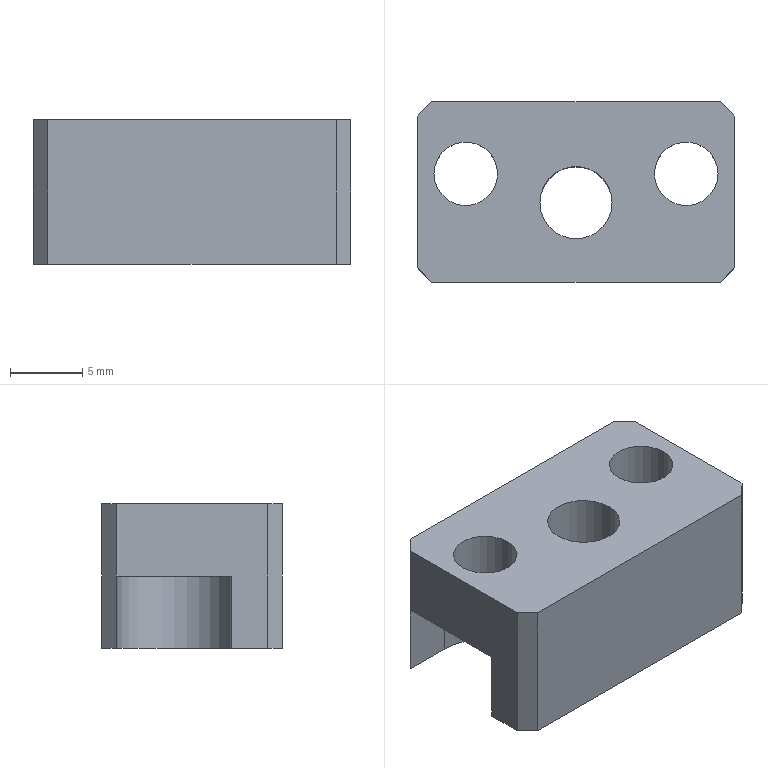Part | SolidWorks | features HoleWzd 2, ICE 2, Chamfer 1, Extrusion 1, MoveFace 1 | 1 solid | 25 faces | box 22 x 12.5 x 10 mm | volume 1861 mm3 | plane 16 | cylinder 9 | commonest cylinder face diameters 4.4 x4 8 x3 5 x2
STEP:
#1=CARTESIAN_POINT('',(5.43,0.,10.));
#2=VERTEX_POINT('',#1);
#3=CARTESIAN_POINT('',(9.83,0.,10.));
#4=VERTEX_POINT('',#3);
#5=CARTESIAN_POINT('',(7.63,0.,10.));
#6=DIRECTION('',(0.,0.,1.));
#7=DIRECTION('',(1.,0.,0.));
#8=AXIS2_PLACEMENT_3D('',#5,#6,#7);
#9=CIRCLE('',#8,2.2);
#10=EDGE_CURVE('',#2,#4,#9,.T.);
#11=ORIENTED_EDGE('',*,*,#10,.T.);
#12=CARTESIAN_POINT('',(9.83,0.,5.));
#13=VERTEX_POINT('',#12);
#14=CARTESIAN_POINT('',(9.83,0.,0.));
#15=DIRECTION('',(0.,0.,-1.));
#16=VECTOR('',#15,1000.);
#17=LINE('',#14,#16);
#18=EDGE_CURVE('',#4,#13,#17,.T.);
#19=ORIENTED_EDGE('',*,*,#18,.T.);
#20=CARTESIAN_POINT('',(5.43,0.,5.));
#21=VERTEX_POINT('',#20);
#22=CARTESIAN_POINT('',(7.63,0.,5.));
#23=DIRECTION('',(0.,0.,-1.));
#24=DIRECTION('',(-1.,0.,0.));
#25=AXIS2_PLACEMENT_3D('',#22,#23,#24);
#26=CIRCLE('',#25,2.2);
#27=EDGE_CURVE('',#13,#21,#26,.T.);
#28=ORIENTED_EDGE('',*,*,#27,.T.);
#29=CARTESIAN_POINT('',(5.43,0.,0.));
#30=DIRECTION('',(0.,0.,-1.));
#31=VECTOR('',#30,1000.);
#32=LINE('',#29,#31);
#33=EDGE_CURVE('',#2,#21,#32,.T.);
#34=ORIENTED_EDGE('',*,*,#33,.F.);
#35=EDGE_LOOP('',(#11,#19,#28,#34));
#36=FACE_OUTER_BOUND('',#35,.T.);
#37=CARTESIAN_POINT('',(7.63,0.,0.));
#38=DIRECTION('',(0.,0.,-1.));
#39=DIRECTION('',(-1.,0.,0.));
#40=AXIS2_PLACEMENT_3D('',#37,#38,#39);
#41=CYLINDRICAL_SURFACE('',#40,2.2);
#42=ADVANCED_FACE('',(#36),#41,.F.);
#43=CARTESIAN_POINT('',(-9.83,0.,10.));
#44=VERTEX_POINT('',#43);
#45=CARTESIAN_POINT('',(-5.43,0.,10.));
#46=VERTEX_POINT('',#45);
#47=CARTESIAN_POINT('',(-7.63,0.,10.));
#48=DIRECTION('',(0.,0.,1.));
#49=DIRECTION('',(1.,0.,0.));
#50=AXIS2_PLACEMENT_3D('',#47,#48,#49);
#51=CIRCLE('',#50,2.2);
#52=EDGE_CURVE('',#44,#46,#51,.T.);
#53=ORIENTED_EDGE('',*,*,#52,.T.);
#54=CARTESIAN_POINT('',(-5.43,0.,5.));
#55=VERTEX_POINT('',#54);
#56=CARTESIAN_POINT('',(-5.43,0.,0.));
#57=DIRECTION('',(0.,0.,-1.));
#58=VECTOR('',#57,1000.);
#59=LINE('',#56,#58);
#60=EDGE_CURVE('',#46,#55,#59,.T.);
#61=ORIENTED_EDGE('',*,*,#60,.T.);
#62=CARTESIAN_POINT('',(-9.83,0.,5.));
#63=VERTEX_POINT('',#62);
#64=CARTESIAN_POINT('',(-7.63,0.,5.));
#65=DIRECTION('',(0.,0.,-1.));
#66=DIRECTION('',(-1.,0.,0.));
#67=AXIS2_PLACEMENT_3D('',#64,#65,#66);
#68=CIRCLE('',#67,2.2);
#69=EDGE_CURVE('',#55,#63,#68,.T.);
#70=ORIENTED_EDGE('',*,*,#69,.T.);
#71=CARTESIAN_POINT('',(-9.83,0.,0.));
#72=DIRECTION('',(0.,0.,-1.));
#73=VECTOR('',#72,1000.);
#74=LINE('',#71,#73);
#75=EDGE_CURVE('',#44,#63,#74,.T.);
#76=ORIENTED_EDGE('',*,*,#75,.F.);
#77=EDGE_LOOP('',(#53,#61,#70,#76));
#78=FACE_OUTER_BOUND('',#77,.T.);
#79=CARTESIAN_POINT('',(-7.63,0.,0.));
#80=DIRECTION('',(0.,0.,-1.));
#81=DIRECTION('',(-1.,0.,0.));
#82=AXIS2_PLACEMENT_3D('',#79,#80,#81);
#83=CYLINDRICAL_SURFACE('',#82,2.2);
#84=ADVANCED_FACE('',(#78),#83,.F.);
#85=CARTESIAN_POINT('',(-2.5,-2.,0.));
#86=VERTEX_POINT('',#85);
#87=CARTESIAN_POINT('',(2.5,-2.,0.));
#88=VERTEX_POINT('',#87);
#89=CARTESIAN_POINT('',(0.,-2.,0.));
#90=DIRECTION('',(0.,0.,1.));
#91=DIRECTION('',(1.,0.,0.));
#92=AXIS2_PLACEMENT_3D('',#89,#90,#91);
#93=CIRCLE('',#92,2.5);
#94=EDGE_CURVE('',#86,#88,#93,.T.);
#95=ORIENTED_EDGE('',*,*,#94,.F.);
#96=CARTESIAN_POINT('',(-2.5,-2.,10.));
#97=VERTEX_POINT('',#96);
#98=CARTESIAN_POINT('',(-2.5,-2.,10.));
#99=DIRECTION('',(0.,0.,1.));
#100=VECTOR('',#99,1000.);
#101=LINE('',#98,#100);
#102=EDGE_CURVE('',#86,#97,#101,.T.);
#103=ORIENTED_EDGE('',*,*,#102,.T.);
#104=CARTESIAN_POINT('',(2.5,-2.,10.));
#105=VERTEX_POINT('',#104);
#106=CARTESIAN_POINT('',(0.,-2.,10.));
#107=DIRECTION('',(0.,0.,1.));
#108=DIRECTION('',(1.,0.,0.));
#109=AXIS2_PLACEMENT_3D('',#106,#107,#108);
#110=CIRCLE('',#109,2.5);
#111=EDGE_CURVE('',#97,#105,#110,.T.);
#112=ORIENTED_EDGE('',*,*,#111,.T.);
#113=CARTESIAN_POINT('',(2.5,-2.,10.));
#114=DIRECTION('',(0.,0.,1.));
#115=VECTOR('',#114,1000.);
#116=LINE('',#113,#115);
#117=EDGE_CURVE('',#88,#105,#116,.T.);
#118=ORIENTED_EDGE('',*,*,#117,.F.);
#119=EDGE_LOOP('',(#95,#103,#112,#118));
#120=FACE_OUTER_BOUND('',#119,.T.);
#121=CARTESIAN_POINT('',(0.,-2.,10.));
#122=DIRECTION('',(0.,0.,1.));
#123=DIRECTION('',(1.,0.,0.));
#124=AXIS2_PLACEMENT_3D('',#121,#122,#123);
#125=CYLINDRICAL_SURFACE('',#124,2.5);
#126=ADVANCED_FACE('',(#120),#125,.F.);
#127=CARTESIAN_POINT('',(3.63,0.,5.));
#128=VERTEX_POINT('',#127);
#129=CARTESIAN_POINT('',(7.63,4.,5.));
#130=VERTEX_POINT('',#129);
#131=CARTESIAN_POINT('',(7.63,0.,5.));
#132=DIRECTION('',(0.,0.,-1.));
#133=DIRECTION('',(-1.,0.,0.));
#134=AXIS2_PLACEMENT_3D('',#131,#132,#133);
#135=CIRCLE('',#134,4.);
#136=EDGE_CURVE('',#128,#130,#135,.T.);
#137=ORIENTED_EDGE('',*,*,#136,.F.);
#138=CARTESIAN_POINT('',(3.63,0.,0.));
#139=VERTEX_POINT('',#138);
#140=CARTESIAN_POINT('',(3.63,0.,0.));
#141=DIRECTION('',(0.,0.,-1.));
#142=VECTOR('',#141,1000.);
#143=LINE('',#140,#142);
#144=EDGE_CURVE('',#128,#139,#143,.T.);
#145=ORIENTED_EDGE('',*,*,#144,.T.);
#146=CARTESIAN_POINT('',(7.63,4.,0.));
#147=VERTEX_POINT('',#146);
#148=CARTESIAN_POINT('',(7.63,0.,0.));
#149=DIRECTION('',(0.,0.,-1.));
#150=DIRECTION('',(-1.,0.,0.));
#151=AXIS2_PLACEMENT_3D('',#148,#149,#150);
#152=CIRCLE('',#151,4.);
#153=EDGE_CURVE('',#139,#147,#152,.T.);
#154=ORIENTED_EDGE('',*,*,#153,.T.);
#155=CARTESIAN_POINT('',(7.63,4.,22.148));
#156=DIRECTION('',(0.,0.,-1.));
#157=VECTOR('',#156,1000.);
#158=LINE('',#155,#157);
#159=EDGE_CURVE('',#130,#147,#158,.T.);
#160=ORIENTED_EDGE('',*,*,#159,.F.);
#161=EDGE_LOOP('',(#137,#145,#154,#160));
#162=FACE_OUTER_BOUND('',#161,.T.);
#163=CARTESIAN_POINT('',(7.63,0.,0.));
#164=DIRECTION('',(0.,0.,-1.));
#165=DIRECTION('',(-1.,0.,0.));
#166=AXIS2_PLACEMENT_3D('',#163,#164,#165);
#167=CYLINDRICAL_SURFACE('',#166,4.);
#168=ADVANCED_FACE('',(#162),#167,.F.);
#169=CARTESIAN_POINT('',(-7.63,4.,0.));
#170=VERTEX_POINT('',#169);
#171=CARTESIAN_POINT('',(-7.63,-4.,0.));
#172=VERTEX_POINT('',#171);
#173=CARTESIAN_POINT('',(-7.63,0.,0.));
#174=DIRECTION('',(0.,0.,-1.));
#175=DIRECTION('',(-1.,0.,0.));
#176=AXIS2_PLACEMENT_3D('',#173,#174,#175);
#177=CIRCLE('',#176,4.);
#178=EDGE_CURVE('',#170,#172,#177,.T.);
#179=ORIENTED_EDGE('',*,*,#178,.T.);
#180=CARTESIAN_POINT('',(-7.63,-4.,5.));
#181=VERTEX_POINT('',#180);
#182=CARTESIAN_POINT('',(-7.63,-4.,22.148));
#183=DIRECTION('',(0.,0.,-1.));
#184=VECTOR('',#183,1000.);
#185=LINE('',#182,#184);
#186=EDGE_CURVE('',#181,#172,#185,.T.);
#187=ORIENTED_EDGE('',*,*,#186,.F.);
#188=CARTESIAN_POINT('',(-7.63,4.,5.));
#189=VERTEX_POINT('',#188);
#190=CARTESIAN_POINT('',(-7.63,0.,5.));
#191=DIRECTION('',(0.,0.,-1.));
#192=DIRECTION('',(-1.,0.,0.));
#193=AXIS2_PLACEMENT_3D('',#190,#191,#192);
#194=CIRCLE('',#193,4.);
#195=EDGE_CURVE('',#189,#181,#194,.T.);
#196=ORIENTED_EDGE('',*,*,#195,.F.);
#197=CARTESIAN_POINT('',(-7.63,4.,22.148));
#198=DIRECTION('',(0.,0.,-1.));
#199=VECTOR('',#198,1000.);
#200=LINE('',#197,#199);
#201=EDGE_CURVE('',#189,#170,#200,.T.);
#202=ORIENTED_EDGE('',*,*,#201,.T.);
#203=EDGE_LOOP('',(#179,#187,#196,#202));
#204=FACE_OUTER_BOUND('',#203,.T.);
#205=CARTESIAN_POINT('',(-7.63,0.,0.));
#206=DIRECTION('',(0.,0.,-1.));
#207=DIRECTION('',(-1.,0.,0.));
#208=AXIS2_PLACEMENT_3D('',#205,#206,#207);
#209=CYLINDRICAL_SURFACE('',#208,4.);
#210=ADVANCED_FACE('',(#204),#209,.F.);
#211=ORIENTED_EDGE('',*,*,#144,.F.);
#212=CARTESIAN_POINT('',(7.63,-4.,5.));
#213=VERTEX_POINT('',#212);
#214=CARTESIAN_POINT('',(7.63,0.,5.));
#215=DIRECTION('',(0.,0.,-1.));
#216=DIRECTION('',(-1.,0.,0.));
#217=AXIS2_PLACEMENT_3D('',#214,#215,#216);
#218=CIRCLE('',#217,4.);
#219=EDGE_CURVE('',#213,#128,#218,.T.);
#220=ORIENTED_EDGE('',*,*,#219,.F.);
#221=CARTESIAN_POINT('',(7.63,-4.,0.));
#222=VERTEX_POINT('',#221);
#223=CARTESIAN_POINT('',(7.63,-4.,22.148));
#224=DIRECTION('',(0.,0.,-1.));
#225=VECTOR('',#224,1000.);
#226=LINE('',#223,#225);
#227=EDGE_CURVE('',#213,#222,#226,.T.);
#228=ORIENTED_EDGE('',*,*,#227,.T.);
#229=CARTESIAN_POINT('',(7.63,0.,0.));
#230=DIRECTION('',(0.,0.,-1.));
#231=DIRECTION('',(-1.,0.,0.));
#232=AXIS2_PLACEMENT_3D('',#229,#230,#231);
#233=CIRCLE('',#232,4.);
#234=EDGE_CURVE('',#222,#139,#233,.T.);
#235=ORIENTED_EDGE('',*,*,#234,.T.);
#236=EDGE_LOOP('',(#211,#220,#228,#235));
#237=FACE_OUTER_BOUND('',#236,.T.);
#238=CARTESIAN_POINT('',(7.63,0.,0.));
#239=DIRECTION('',(0.,0.,-1.));
#240=DIRECTION('',(-1.,0.,0.));
#241=AXIS2_PLACEMENT_3D('',#238,#239,#240);
#242=CYLINDRICAL_SURFACE('',#241,4.);
#243=ADVANCED_FACE('',(#237),#242,.F.);
#244=CARTESIAN_POINT('',(0.,-2.,0.));
#245=DIRECTION('',(0.,0.,1.));
#246=DIRECTION('',(1.,0.,0.));
#247=AXIS2_PLACEMENT_3D('',#244,#245,#246);
#248=CIRCLE('',#247,2.5);
#249=EDGE_CURVE('',#88,#86,#248,.T.);
#250=ORIENTED_EDGE('',*,*,#249,.T.);
#251=ORIENTED_EDGE('',*,*,#94,.T.);
#252=EDGE_LOOP('',(#250,#251));
#253=FACE_BOUND('',#252,.T.);
#254=CARTESIAN_POINT('',(-11.,-4.,0.));
#255=VERTEX_POINT('',#254);
#256=CARTESIAN_POINT('',(-11.,-6.5,0.));
#257=VERTEX_POINT('',#256);
#258=CARTESIAN_POINT('',(-11.,7.5,0.));
#259=DIRECTION('',(0.,-1.,0.));
#260=VECTOR('',#259,1000.);
#261=LINE('',#258,#260);
#262=EDGE_CURVE('',#255,#257,#261,.T.);
#263=ORIENTED_EDGE('',*,*,#262,.F.);
#264=CARTESIAN_POINT('',(-7.63,-4.,0.));
#265=DIRECTION('',(-1.,0.,0.));
#266=VECTOR('',#265,1000.);
#267=LINE('',#264,#266);
#268=EDGE_CURVE('',#172,#255,#267,.T.);
#269=ORIENTED_EDGE('',*,*,#268,.F.);
#270=ORIENTED_EDGE('',*,*,#178,.F.);
#271=CARTESIAN_POINT('',(-11.,4.,0.));
#272=VERTEX_POINT('',#271);
#273=CARTESIAN_POINT('',(-7.63,4.,0.));
#274=DIRECTION('',(1.,0.,0.));
#275=VECTOR('',#274,1000.);
#276=LINE('',#273,#275);
#277=EDGE_CURVE('',#272,#170,#276,.T.);
#278=ORIENTED_EDGE('',*,*,#277,.F.);
#279=CARTESIAN_POINT('',(-10.,5.,0.));
#280=VERTEX_POINT('',#279);
#281=CARTESIAN_POINT('',(-11.,4.,0.));
#282=DIRECTION('',(0.7071,0.7071,0.));
#283=VECTOR('',#282,1000.);
#284=LINE('',#281,#283);
#285=EDGE_CURVE('',#272,#280,#284,.T.);
#286=ORIENTED_EDGE('',*,*,#285,.T.);
#287=CARTESIAN_POINT('',(10.,5.,0.));
#288=VERTEX_POINT('',#287);
#289=CARTESIAN_POINT('',(-11.,5.,0.));
#290=DIRECTION('',(-1.,0.,0.));
#291=VECTOR('',#290,1000.);
#292=LINE('',#289,#291);
#293=EDGE_CURVE('',#288,#280,#292,.T.);
#294=ORIENTED_EDGE('',*,*,#293,.F.);
#295=CARTESIAN_POINT('',(11.,4.,0.));
#296=VERTEX_POINT('',#295);
#297=CARTESIAN_POINT('',(11.,4.,0.));
#298=DIRECTION('',(0.7071,-0.7071,0.));
#299=VECTOR('',#298,1000.);
#300=LINE('',#297,#299);
#301=EDGE_CURVE('',#288,#296,#300,.T.);
#302=ORIENTED_EDGE('',*,*,#301,.T.);
#303=CARTESIAN_POINT('',(7.63,4.,0.));
#304=DIRECTION('',(1.,0.,0.));
#305=VECTOR('',#304,1000.);
#306=LINE('',#303,#305);
#307=EDGE_CURVE('',#147,#296,#306,.T.);
#308=ORIENTED_EDGE('',*,*,#307,.F.);
#309=ORIENTED_EDGE('',*,*,#153,.F.);
#310=ORIENTED_EDGE('',*,*,#234,.F.);
#311=CARTESIAN_POINT('',(11.,-4.,0.));
#312=VERTEX_POINT('',#311);
#313=CARTESIAN_POINT('',(7.63,-4.,0.));
#314=DIRECTION('',(-1.,0.,0.));
#315=VECTOR('',#314,1000.);
#316=LINE('',#313,#315);
#317=EDGE_CURVE('',#312,#222,#316,.T.);
#318=ORIENTED_EDGE('',*,*,#317,.F.);
#319=CARTESIAN_POINT('',(11.,-6.5,0.));
#320=VERTEX_POINT('',#319);
#321=CARTESIAN_POINT('',(11.,7.5,0.));
#322=DIRECTION('',(0.,1.,0.));
#323=VECTOR('',#322,1000.);
#324=LINE('',#321,#323);
#325=EDGE_CURVE('',#320,#312,#324,.T.);
#326=ORIENTED_EDGE('',*,*,#325,.F.);
#327=CARTESIAN_POINT('',(10.,-7.5,0.));
#328=VERTEX_POINT('',#327);
#329=CARTESIAN_POINT('',(11.,-6.5,0.));
#330=DIRECTION('',(-0.7071,-0.7071,0.));
#331=VECTOR('',#330,1000.);
#332=LINE('',#329,#331);
#333=EDGE_CURVE('',#320,#328,#332,.T.);
#334=ORIENTED_EDGE('',*,*,#333,.T.);
#335=CARTESIAN_POINT('',(-10.,-7.5,0.));
#336=VERTEX_POINT('',#335);
#337=CARTESIAN_POINT('',(-11.,-7.5,0.));
#338=DIRECTION('',(1.,0.,0.));
#339=VECTOR('',#338,1000.);
#340=LINE('',#337,#339);
#341=EDGE_CURVE('',#336,#328,#340,.T.);
#342=ORIENTED_EDGE('',*,*,#341,.F.);
#343=CARTESIAN_POINT('',(-10.,-7.5,0.));
#344=DIRECTION('',(-0.7071,0.7071,0.));
#345=VECTOR('',#344,1000.);
#346=LINE('',#343,#345);
#347=EDGE_CURVE('',#336,#257,#346,.T.);
#348=ORIENTED_EDGE('',*,*,#347,.T.);
#349=EDGE_LOOP('',(#263,#269,#270,#278,#286,#294,#302,#308,#309,#310,#318,#326,#334,#342,#348));
#350=FACE_OUTER_BOUND('',#349,.T.);
#351=CARTESIAN_POINT('',(0.,0.,0.));
#352=DIRECTION('',(0.,0.,1.));
#353=DIRECTION('',(1.,0.,0.));
#354=AXIS2_PLACEMENT_3D('',#351,#352,#353);
#355=PLANE('',#354);
#356=ADVANCED_FACE('',(#253,#350),#355,.F.);
#357=CARTESIAN_POINT('',(11.,-4.,5.));
#358=VERTEX_POINT('',#357);
#359=CARTESIAN_POINT('',(11.,4.,5.));
#360=VERTEX_POINT('',#359);
#361=CARTESIAN_POINT('',(11.,7.5,5.));
#362=DIRECTION('',(0.,1.,0.));
#363=VECTOR('',#362,1000.);
#364=LINE('',#361,#363);
#365=EDGE_CURVE('',#358,#360,#364,.T.);
#366=ORIENTED_EDGE('',*,*,#365,.T.);
#367=CARTESIAN_POINT('',(11.,4.,10.));
#368=VERTEX_POINT('',#367);
#369=CARTESIAN_POINT('',(11.,4.,10.));
#370=DIRECTION('',(0.,0.,1.));
#371=VECTOR('',#370,1000.);
#372=LINE('',#369,#371);
#373=EDGE_CURVE('',#360,#368,#372,.T.);
#374=ORIENTED_EDGE('',*,*,#373,.T.);
#375=CARTESIAN_POINT('',(11.,-6.5,10.));
#376=VERTEX_POINT('',#375);
#377=CARTESIAN_POINT('',(11.,7.5,10.));
#378=DIRECTION('',(0.,1.,0.));
#379=VECTOR('',#378,1000.);
#380=LINE('',#377,#379);
#381=EDGE_CURVE('',#376,#368,#380,.T.);
#382=ORIENTED_EDGE('',*,*,#381,.F.);
#383=CARTESIAN_POINT('',(11.,-6.5,10.));
#384=DIRECTION('',(0.,0.,-1.));
#385=VECTOR('',#384,1000.);
#386=LINE('',#383,#385);
#387=EDGE_CURVE('',#376,#320,#386,.T.);
#388=ORIENTED_EDGE('',*,*,#387,.T.);
#389=ORIENTED_EDGE('',*,*,#325,.T.);
#390=CARTESIAN_POINT('',(11.,-4.,10.));
#391=DIRECTION('',(0.,0.,1.));
#392=VECTOR('',#391,1000.);
#393=LINE('',#390,#392);
#394=EDGE_CURVE('',#312,#358,#393,.T.);
#395=ORIENTED_EDGE('',*,*,#394,.T.);
#396=EDGE_LOOP('',(#366,#374,#382,#388,#389,#395));
#397=FACE_OUTER_BOUND('',#396,.T.);
#398=CARTESIAN_POINT('',(11.,7.5,10.));
#399=DIRECTION('',(-1.,0.,0.));
#400=DIRECTION('',(0.,0.,1.));
#401=AXIS2_PLACEMENT_3D('',#398,#399,#400);
#402=PLANE('',#401);
#403=ADVANCED_FACE('',(#397),#402,.F.);
#404=CARTESIAN_POINT('',(-11.,4.,10.));
#405=VERTEX_POINT('',#404);
#406=CARTESIAN_POINT('',(-11.,4.,5.));
#407=VERTEX_POINT('',#406);
#408=CARTESIAN_POINT('',(-11.,4.,10.));
#409=DIRECTION('',(0.,0.,-1.));
#410=VECTOR('',#409,1000.);
#411=LINE('',#408,#410);
#412=EDGE_CURVE('',#405,#407,#411,.T.);
#413=ORIENTED_EDGE('',*,*,#412,.T.);
#414=CARTESIAN_POINT('',(-11.,-4.,5.));
#415=VERTEX_POINT('',#414);
#416=CARTESIAN_POINT('',(-11.,7.5,5.));
#417=DIRECTION('',(0.,-1.,0.));
#418=VECTOR('',#417,1000.);
#419=LINE('',#416,#418);
#420=EDGE_CURVE('',#407,#415,#419,.T.);
#421=ORIENTED_EDGE('',*,*,#420,.T.);
#422=CARTESIAN_POINT('',(-11.,-4.,10.));
#423=DIRECTION('',(0.,0.,-1.));
#424=VECTOR('',#423,1000.);
#425=LINE('',#422,#424);
#426=EDGE_CURVE('',#415,#255,#425,.T.);
#427=ORIENTED_EDGE('',*,*,#426,.T.);
#428=ORIENTED_EDGE('',*,*,#262,.T.);
#429=CARTESIAN_POINT('',(-11.,-6.5,10.));
#430=VERTEX_POINT('',#429);
#431=CARTESIAN_POINT('',(-11.,-6.5,10.));
#432=DIRECTION('',(0.,0.,1.));
#433=VECTOR('',#432,1000.);
#434=LINE('',#431,#433);
#435=EDGE_CURVE('',#257,#430,#434,.T.);
#436=ORIENTED_EDGE('',*,*,#435,.T.);
#437=CARTESIAN_POINT('',(-11.,7.5,10.));
#438=DIRECTION('',(0.,-1.,0.));
#439=VECTOR('',#438,1000.);
#440=LINE('',#437,#439);
#441=EDGE_CURVE('',#405,#430,#440,.T.);
#442=ORIENTED_EDGE('',*,*,#441,.F.);
#443=EDGE_LOOP('',(#413,#421,#427,#428,#436,#442));
#444=FACE_OUTER_BOUND('',#443,.T.);
#445=CARTESIAN_POINT('',(-11.,7.5,10.));
#446=DIRECTION('',(1.,0.,0.));
#447=DIRECTION('',(0.,1.,0.));
#448=AXIS2_PLACEMENT_3D('',#445,#446,#447);
#449=PLANE('',#448);
#450=ADVANCED_FACE('',(#444),#449,.F.);
#451=CARTESIAN_POINT('',(-10.,-7.5,10.));
#452=VERTEX_POINT('',#451);
#453=CARTESIAN_POINT('',(10.,-7.5,10.));
#454=VERTEX_POINT('',#453);
#455=CARTESIAN_POINT('',(-11.,-7.5,10.));
#456=DIRECTION('',(1.,0.,0.));
#457=VECTOR('',#456,1000.);
#458=LINE('',#455,#457);
#459=EDGE_CURVE('',#452,#454,#458,.T.);
#460=ORIENTED_EDGE('',*,*,#459,.F.);
#461=CARTESIAN_POINT('',(-10.,-7.5,10.));
#462=DIRECTION('',(0.,0.,-1.));
#463=VECTOR('',#462,1000.);
#464=LINE('',#461,#463);
#465=EDGE_CURVE('',#452,#336,#464,.T.);
#466=ORIENTED_EDGE('',*,*,#465,.T.);
#467=ORIENTED_EDGE('',*,*,#341,.T.);
#468=CARTESIAN_POINT('',(10.,-7.5,10.));
#469=DIRECTION('',(0.,0.,1.));
#470=VECTOR('',#469,1000.);
#471=LINE('',#468,#470);
#472=EDGE_CURVE('',#328,#454,#471,.T.);
#473=ORIENTED_EDGE('',*,*,#472,.T.);
#474=EDGE_LOOP('',(#460,#466,#467,#473));
#475=FACE_OUTER_BOUND('',#474,.T.);
#476=CARTESIAN_POINT('',(-11.,-7.5,10.));
#477=DIRECTION('',(0.,1.,0.));
#478=DIRECTION('',(0.,0.,1.));
#479=AXIS2_PLACEMENT_3D('',#476,#477,#478);
#480=PLANE('',#479);
#481=ADVANCED_FACE('',(#475),#480,.F.);
#482=CARTESIAN_POINT('',(-10.,5.,10.));
#483=VERTEX_POINT('',#482);
#484=CARTESIAN_POINT('',(10.,5.,10.));
#485=VERTEX_POINT('',#484);
#486=CARTESIAN_POINT('',(0.,5.,10.));
#487=DIRECTION('',(1.,0.,0.));
#488=VECTOR('',#487,1000.);
#489=LINE('',#486,#488);
#490=EDGE_CURVE('',#483,#485,#489,.T.);
#491=ORIENTED_EDGE('',*,*,#490,.F.);
#492=CARTESIAN_POINT('',(-7.5,7.5,10.));
#493=DIRECTION('',(-0.7071,-0.7071,0.));
#494=VECTOR('',#493,1000.);
#495=LINE('',#492,#494);
#496=EDGE_CURVE('',#483,#405,#495,.T.);
#497=ORIENTED_EDGE('',*,*,#496,.T.);
#498=ORIENTED_EDGE('',*,*,#441,.T.);
#499=CARTESIAN_POINT('',(-8.75,-8.75,10.));
#500=DIRECTION('',(0.7071,-0.7071,0.));
#501=VECTOR('',#500,1000.);
#502=LINE('',#499,#501);
#503=EDGE_CURVE('',#430,#452,#502,.T.);
#504=ORIENTED_EDGE('',*,*,#503,.T.);
#505=ORIENTED_EDGE('',*,*,#459,.T.);
#506=CARTESIAN_POINT('',(8.75,-8.75,10.));
#507=DIRECTION('',(0.7071,0.7071,0.));
#508=VECTOR('',#507,1000.);
#509=LINE('',#506,#508);
#510=EDGE_CURVE('',#454,#376,#509,.T.);
#511=ORIENTED_EDGE('',*,*,#510,.T.);
#512=ORIENTED_EDGE('',*,*,#381,.T.);
#513=CARTESIAN_POINT('',(7.5,7.5,10.));
#514=DIRECTION('',(-0.7071,0.7071,0.));
#515=VECTOR('',#514,1000.);
#516=LINE('',#513,#515);
#517=EDGE_CURVE('',#368,#485,#516,.T.);
#518=ORIENTED_EDGE('',*,*,#517,.T.);
#519=EDGE_LOOP('',(#491,#497,#498,#504,#505,#511,#512,#518));
#520=FACE_OUTER_BOUND('',#519,.T.);
#521=ORIENTED_EDGE('',*,*,#10,.F.);
#522=CARTESIAN_POINT('',(7.63,0.,10.));
#523=DIRECTION('',(0.,0.,1.));
#524=DIRECTION('',(1.,0.,0.));
#525=AXIS2_PLACEMENT_3D('',#522,#523,#524);
#526=CIRCLE('',#525,2.2);
#527=EDGE_CURVE('',#4,#2,#526,.T.);
#528=ORIENTED_EDGE('',*,*,#527,.F.);
#529=EDGE_LOOP('',(#521,#528));
#530=FACE_BOUND('',#529,.T.);
#531=ORIENTED_EDGE('',*,*,#52,.F.);
#532=CARTESIAN_POINT('',(-7.63,0.,10.));
#533=DIRECTION('',(0.,0.,1.));
#534=DIRECTION('',(1.,0.,0.));
#535=AXIS2_PLACEMENT_3D('',#532,#533,#534);
#536=CIRCLE('',#535,2.2);
#537=EDGE_CURVE('',#46,#44,#536,.T.);
#538=ORIENTED_EDGE('',*,*,#537,.F.);
#539=EDGE_LOOP('',(#531,#538));
#540=FACE_BOUND('',#539,.T.);
#541=CARTESIAN_POINT('',(0.,-2.,10.));
#542=DIRECTION('',(0.,0.,1.));
#543=DIRECTION('',(1.,0.,0.));
#544=AXIS2_PLACEMENT_3D('',#541,#542,#543);
#545=CIRCLE('',#544,2.5);
#546=EDGE_CURVE('',#105,#97,#545,.T.);
#547=ORIENTED_EDGE('',*,*,#546,.F.);
#548=ORIENTED_EDGE('',*,*,#111,.F.);
#549=EDGE_LOOP('',(#547,#548));
#550=FACE_BOUND('',#549,.T.);
#551=CARTESIAN_POINT('',(0.,0.,10.));
#552=DIRECTION('',(0.,0.,1.));
#553=DIRECTION('',(1.,0.,0.));
#554=AXIS2_PLACEMENT_3D('',#551,#552,#553);
#555=PLANE('',#554);
#556=ADVANCED_FACE('',(#520,#530,#540,#550),#555,.T.);
#557=ORIENTED_EDGE('',*,*,#102,.F.);
#558=ORIENTED_EDGE('',*,*,#249,.F.);
#559=ORIENTED_EDGE('',*,*,#117,.T.);
#560=ORIENTED_EDGE('',*,*,#546,.T.);
#561=EDGE_LOOP('',(#557,#558,#559,#560));
#562=FACE_OUTER_BOUND('',#561,.T.);
#563=CARTESIAN_POINT('',(0.,-2.,10.));
#564=DIRECTION('',(0.,0.,1.));
#565=DIRECTION('',(1.,0.,0.));
#566=AXIS2_PLACEMENT_3D('',#563,#564,#565);
#567=CYLINDRICAL_SURFACE('',#566,2.5);
#568=ADVANCED_FACE('',(#562),#567,.F.);
#569=CARTESIAN_POINT('',(-7.63,0.,5.));
#570=DIRECTION('',(0.,0.,-1.));
#571=DIRECTION('',(-1.,0.,0.));
#572=AXIS2_PLACEMENT_3D('',#569,#570,#571);
#573=CIRCLE('',#572,2.2);
#574=EDGE_CURVE('',#63,#55,#573,.T.);
#575=ORIENTED_EDGE('',*,*,#574,.F.);
#576=ORIENTED_EDGE('',*,*,#69,.F.);
#577=EDGE_LOOP('',(#575,#576));
#578=FACE_BOUND('',#577,.T.);
#579=ORIENTED_EDGE('',*,*,#420,.F.);
#580=CARTESIAN_POINT('',(-7.63,4.,5.));
#581=DIRECTION('',(1.,0.,0.));
#582=VECTOR('',#581,1000.);
#583=LINE('',#580,#582);
#584=EDGE_CURVE('',#407,#189,#583,.T.);
#585=ORIENTED_EDGE('',*,*,#584,.T.);
#586=ORIENTED_EDGE('',*,*,#195,.T.);
#587=CARTESIAN_POINT('',(-7.63,-4.,5.));
#588=DIRECTION('',(-1.,0.,0.));
#589=VECTOR('',#588,1000.);
#590=LINE('',#587,#589);
#591=EDGE_CURVE('',#181,#415,#590,.T.);
#592=ORIENTED_EDGE('',*,*,#591,.T.);
#593=EDGE_LOOP('',(#579,#585,#586,#592));
#594=FACE_OUTER_BOUND('',#593,.T.);
#595=CARTESIAN_POINT('',(-5.43,0.,5.));
#596=DIRECTION('',(0.,0.,1.));
#597=DIRECTION('',(1.,0.,0.));
#598=AXIS2_PLACEMENT_3D('',#595,#596,#597);
#599=PLANE('',#598);
#600=ADVANCED_FACE('',(#578,#594),#599,.F.);
#601=ORIENTED_EDGE('',*,*,#60,.F.);
#602=ORIENTED_EDGE('',*,*,#537,.T.);
#603=ORIENTED_EDGE('',*,*,#75,.T.);
#604=ORIENTED_EDGE('',*,*,#574,.T.);
#605=EDGE_LOOP('',(#601,#602,#603,#604));
#606=FACE_OUTER_BOUND('',#605,.T.);
#607=CARTESIAN_POINT('',(-7.63,0.,0.));
#608=DIRECTION('',(0.,0.,-1.));
#609=DIRECTION('',(-1.,0.,0.));
#610=AXIS2_PLACEMENT_3D('',#607,#608,#609);
#611=CYLINDRICAL_SURFACE('',#610,2.2);
#612=ADVANCED_FACE('',(#606),#611,.F.);
#613=CARTESIAN_POINT('',(7.63,0.,5.));
#614=DIRECTION('',(0.,0.,-1.));
#615=DIRECTION('',(-1.,0.,0.));
#616=AXIS2_PLACEMENT_3D('',#613,#614,#615);
#617=CIRCLE('',#616,2.2);
#618=EDGE_CURVE('',#21,#13,#617,.T.);
#619=ORIENTED_EDGE('',*,*,#618,.F.);
#620=ORIENTED_EDGE('',*,*,#27,.F.);
#621=EDGE_LOOP('',(#619,#620));
#622=FACE_BOUND('',#621,.T.);
#623=ORIENTED_EDGE('',*,*,#365,.F.);
#624=CARTESIAN_POINT('',(7.63,-4.,5.));
#625=DIRECTION('',(-1.,0.,0.));
#626=VECTOR('',#625,1000.);
#627=LINE('',#624,#626);
#628=EDGE_CURVE('',#358,#213,#627,.T.);
#629=ORIENTED_EDGE('',*,*,#628,.T.);
#630=ORIENTED_EDGE('',*,*,#219,.T.);
#631=ORIENTED_EDGE('',*,*,#136,.T.);
#632=CARTESIAN_POINT('',(7.63,4.,5.));
#633=DIRECTION('',(1.,0.,0.));
#634=VECTOR('',#633,1000.);
#635=LINE('',#632,#634);
#636=EDGE_CURVE('',#130,#360,#635,.T.);
#637=ORIENTED_EDGE('',*,*,#636,.T.);
#638=EDGE_LOOP('',(#623,#629,#630,#631,#637));
#639=FACE_OUTER_BOUND('',#638,.T.);
#640=CARTESIAN_POINT('',(9.83,0.,5.));
#641=DIRECTION('',(0.,0.,1.));
#642=DIRECTION('',(1.,0.,0.));
#643=AXIS2_PLACEMENT_3D('',#640,#641,#642);
#644=PLANE('',#643);
#645=ADVANCED_FACE('',(#622,#639),#644,.F.);
#646=ORIENTED_EDGE('',*,*,#18,.F.);
#647=ORIENTED_EDGE('',*,*,#527,.T.);
#648=ORIENTED_EDGE('',*,*,#33,.T.);
#649=ORIENTED_EDGE('',*,*,#618,.T.);
#650=EDGE_LOOP('',(#646,#647,#648,#649));
#651=FACE_OUTER_BOUND('',#650,.T.);
#652=CARTESIAN_POINT('',(7.63,0.,0.));
#653=DIRECTION('',(0.,0.,-1.));
#654=DIRECTION('',(-1.,0.,0.));
#655=AXIS2_PLACEMENT_3D('',#652,#653,#654);
#656=CYLINDRICAL_SURFACE('',#655,2.2);
#657=ADVANCED_FACE('',(#651),#656,.F.);
#658=ORIENTED_EDGE('',*,*,#293,.T.);
#659=CARTESIAN_POINT('',(-10.,5.,10.));
#660=DIRECTION('',(0.,0.,1.));
#661=VECTOR('',#660,1000.);
#662=LINE('',#659,#661);
#663=EDGE_CURVE('',#280,#483,#662,.T.);
#664=ORIENTED_EDGE('',*,*,#663,.T.);
#665=ORIENTED_EDGE('',*,*,#490,.T.);
#666=CARTESIAN_POINT('',(10.,5.,10.));
#667=DIRECTION('',(0.,0.,-1.));
#668=VECTOR('',#667,1000.);
#669=LINE('',#666,#668);
#670=EDGE_CURVE('',#485,#288,#669,.T.);
#671=ORIENTED_EDGE('',*,*,#670,.T.);
#672=EDGE_LOOP('',(#658,#664,#665,#671));
#673=FACE_OUTER_BOUND('',#672,.T.);
#674=CARTESIAN_POINT('',(-11.,5.,10.));
#675=DIRECTION('',(0.,-1.,0.));
#676=DIRECTION('',(1.,0.,0.));
#677=AXIS2_PLACEMENT_3D('',#674,#675,#676);
#678=PLANE('',#677);
#679=ADVANCED_FACE('',(#673),#678,.F.);
#680=ORIENTED_EDGE('',*,*,#496,.F.);
#681=ORIENTED_EDGE('',*,*,#663,.F.);
#682=ORIENTED_EDGE('',*,*,#285,.F.);
#683=CARTESIAN_POINT('',(-11.,4.,10.));
#684=DIRECTION('',(0.,0.,-1.));
#685=VECTOR('',#684,1000.);
#686=LINE('',#683,#685);
#687=EDGE_CURVE('',#407,#272,#686,.T.);
#688=ORIENTED_EDGE('',*,*,#687,.F.);
#689=ORIENTED_EDGE('',*,*,#412,.F.);
#690=EDGE_LOOP('',(#680,#681,#682,#688,#689));
#691=FACE_OUTER_BOUND('',#690,.T.);
#692=CARTESIAN_POINT('',(-11.,4.,10.));
#693=DIRECTION('',(0.7071,-0.7071,0.));
#694=DIRECTION('',(0.,0.,-1.));
#695=AXIS2_PLACEMENT_3D('',#692,#693,#694);
#696=PLANE('',#695);
#697=ADVANCED_FACE('',(#691),#696,.F.);
#698=ORIENTED_EDGE('',*,*,#503,.F.);
#699=ORIENTED_EDGE('',*,*,#435,.F.);
#700=ORIENTED_EDGE('',*,*,#347,.F.);
#701=ORIENTED_EDGE('',*,*,#465,.F.);
#702=EDGE_LOOP('',(#698,#699,#700,#701));
#703=FACE_OUTER_BOUND('',#702,.T.);
#704=CARTESIAN_POINT('',(-10.,-7.5,10.));
#705=DIRECTION('',(0.7071,0.7071,0.));
#706=DIRECTION('',(0.,0.,-1.));
#707=AXIS2_PLACEMENT_3D('',#704,#705,#706);
#708=PLANE('',#707);
#709=ADVANCED_FACE('',(#703),#708,.F.);
#710=ORIENTED_EDGE('',*,*,#301,.F.);
#711=ORIENTED_EDGE('',*,*,#670,.F.);
#712=ORIENTED_EDGE('',*,*,#517,.F.);
#713=ORIENTED_EDGE('',*,*,#373,.F.);
#714=CARTESIAN_POINT('',(11.,4.,10.));
#715=DIRECTION('',(0.,0.,1.));
#716=VECTOR('',#715,1000.);
#717=LINE('',#714,#716);
#718=EDGE_CURVE('',#296,#360,#717,.T.);
#719=ORIENTED_EDGE('',*,*,#718,.F.);
#720=EDGE_LOOP('',(#710,#711,#712,#713,#719));
#721=FACE_OUTER_BOUND('',#720,.T.);
#722=CARTESIAN_POINT('',(11.,4.,10.));
#723=DIRECTION('',(-0.7071,-0.7071,0.));
#724=DIRECTION('',(0.,0.,1.));
#725=AXIS2_PLACEMENT_3D('',#722,#723,#724);
#726=PLANE('',#725);
#727=ADVANCED_FACE('',(#721),#726,.F.);
#728=ORIENTED_EDGE('',*,*,#510,.F.);
#729=ORIENTED_EDGE('',*,*,#472,.F.);
#730=ORIENTED_EDGE('',*,*,#333,.F.);
#731=ORIENTED_EDGE('',*,*,#387,.F.);
#732=EDGE_LOOP('',(#728,#729,#730,#731));
#733=FACE_OUTER_BOUND('',#732,.T.);
#734=CARTESIAN_POINT('',(11.,-6.5,10.));
#735=DIRECTION('',(-0.7071,0.7071,0.));
#736=DIRECTION('',(0.,0.,-1.));
#737=AXIS2_PLACEMENT_3D('',#734,#735,#736);
#738=PLANE('',#737);
#739=ADVANCED_FACE('',(#733),#738,.F.);
#740=ORIENTED_EDGE('',*,*,#718,.T.);
#741=ORIENTED_EDGE('',*,*,#636,.F.);
#742=ORIENTED_EDGE('',*,*,#159,.T.);
#743=ORIENTED_EDGE('',*,*,#307,.T.);
#744=EDGE_LOOP('',(#740,#741,#742,#743));
#745=FACE_OUTER_BOUND('',#744,.T.);
#746=CARTESIAN_POINT('',(7.63,4.,22.148));
#747=DIRECTION('',(0.,1.,0.));
#748=DIRECTION('',(-1.,0.,0.));
#749=AXIS2_PLACEMENT_3D('',#746,#747,#748);
#750=PLANE('',#749);
#751=ADVANCED_FACE('',(#745),#750,.F.);
#752=ORIENTED_EDGE('',*,*,#317,.T.);
#753=ORIENTED_EDGE('',*,*,#227,.F.);
#754=ORIENTED_EDGE('',*,*,#628,.F.);
#755=ORIENTED_EDGE('',*,*,#394,.F.);
#756=EDGE_LOOP('',(#752,#753,#754,#755));
#757=FACE_OUTER_BOUND('',#756,.T.);
#758=CARTESIAN_POINT('',(7.63,-4.,22.148));
#759=DIRECTION('',(0.,-1.,0.));
#760=DIRECTION('',(1.,0.,0.));
#761=AXIS2_PLACEMENT_3D('',#758,#759,#760);
#762=PLANE('',#761);
#763=ADVANCED_FACE('',(#757),#762,.F.);
#764=ORIENTED_EDGE('',*,*,#687,.T.);
#765=ORIENTED_EDGE('',*,*,#277,.T.);
#766=ORIENTED_EDGE('',*,*,#201,.F.);
#767=ORIENTED_EDGE('',*,*,#584,.F.);
#768=EDGE_LOOP('',(#764,#765,#766,#767));
#769=FACE_OUTER_BOUND('',#768,.T.);
#770=CARTESIAN_POINT('',(-7.63,4.,22.148));
#771=DIRECTION('',(0.,1.,0.));
#772=DIRECTION('',(-1.,0.,0.));
#773=AXIS2_PLACEMENT_3D('',#770,#771,#772);
#774=PLANE('',#773);
#775=ADVANCED_FACE('',(#769),#774,.F.);
#776=ORIENTED_EDGE('',*,*,#591,.F.);
#777=ORIENTED_EDGE('',*,*,#186,.T.);
#778=ORIENTED_EDGE('',*,*,#268,.T.);
#779=ORIENTED_EDGE('',*,*,#426,.F.);
#780=EDGE_LOOP('',(#776,#777,#778,#779));
#781=FACE_OUTER_BOUND('',#780,.T.);
#782=CARTESIAN_POINT('',(-7.63,-4.,22.148));
#783=DIRECTION('',(0.,-1.,0.));
#784=DIRECTION('',(1.,0.,0.));
#785=AXIS2_PLACEMENT_3D('',#782,#783,#784);
#786=PLANE('',#785);
#787=ADVANCED_FACE('',(#781),#786,.F.);
#788=CLOSED_SHELL('',(#42,#84,#126,#168,#210,#243,#356,#403,#450,#481,#556,#568,#600,#612,#645,#657,#679,#697,#709,#727,#739,#751,#763,#775,#787));
#789=MANIFOLD_SOLID_BREP('',#788);
#790=CARTESIAN_POINT('',(0.,0.,0.));
#791=DIRECTION('',(0.,0.,1.));
#792=DIRECTION('',(1.,0.,0.));
#793=AXIS2_PLACEMENT_3D('',#790,#791,#792);
#794=(LENGTH_UNIT()NAMED_UNIT(*)SI_UNIT(.MILLI.,.METRE.));
#795=UNCERTAINTY_MEASURE_WITH_UNIT(LENGTH_MEASURE(0.00001),#794,'','');
#796=(NAMED_UNIT(*)PLANE_ANGLE_UNIT()SI_UNIT($,.RADIAN.));
#797=(NAMED_UNIT(*)SI_UNIT($,.STERADIAN.)SOLID_ANGLE_UNIT());
#798=(GEOMETRIC_REPRESENTATION_CONTEXT(3)GLOBAL_UNCERTAINTY_ASSIGNED_CONTEXT((#795))GLOBAL_UNIT_ASSIGNED_CONTEXT((#794,#796,#797))REPRESENTATION_CONTEXT('',''));
#799=ADVANCED_BREP_SHAPE_REPRESENTATION('',(#789,#793),#798);